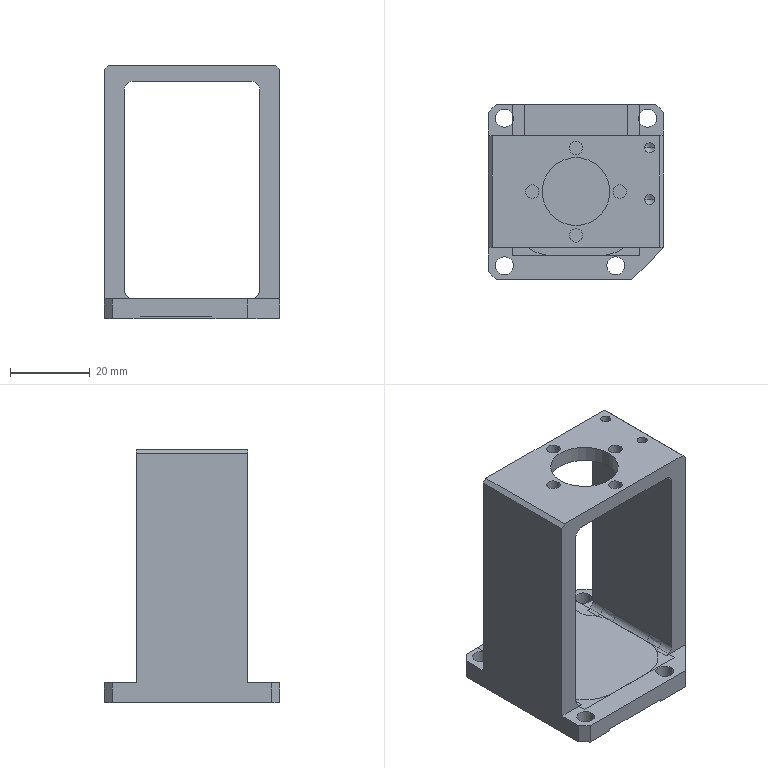NC program | NX | posted with a generic post | part box 44 x 44 x 63.6 mm
Whole program:
N10 G17 G21 G94 G90
(FLOOR_WALL_COPY , TOOL : D63)
N12 T01 M6
N14 G54
N16 G17 G0 G90 X58.5 Y0. B0. C0. S6500 M3
N18 G43 Z30. H1
N20 Z8.
N22 G94 G1 Z5. F1500.
N24 X53.5
N26 X-53.5
N28 X-58.5
N30 Z8.
N32 G0 Z30.
N34 X58.5
N36 Z7.
N38 G1 Z4.
N40 X53.5
N42 X-53.5
N44 X-58.5
N46 Z7.
N48 G0 Z30.
N50 X58.5
N52 Z6.
N54 G1 Z3.
N56 X53.5
N58 X-53.5
N60 X-58.5
N62 Z6.
N64 G0 Z30.
N66 X58.5
N68 Z5.
N70 G1 Z2.
N72 X53.5
N74 X-53.5
N76 X-58.5
N78 Z5.
N80 G0 Z30.
N82 X58.5
N84 Z4.
N86 G1 Z1.
N88 X53.5
N90 X-53.5
N92 X-58.5
N94 Z4.
N96 G0 Z30.
N98 X58.5
N100 Z3.
N102 G1 Z0.
N104 X53.5
N106 X-53.5
N108 X-58.5
N110 Z3.
N112 G0 Z30.
N114 M5
(FLOOR_WALL_1_COPY_1 , TOOL : D10)
N116 T10 M6
N118 G54
N120 G17 G0 G90 X-5.732 Y29. B0. C0. S9500 M3
N122 G43 Z30. H10
N124 Z-0.4
N126 G94 G1 X-4.866 Y27.5 F1000.
N128 G3 X-4. Y27. R1.
N130 G1 X-0.1 F2500.
N132 Y11.
N134 X-6.
N136 G3 X-8.679 Y10.222 R5.
N138 G1 X-8.684 Y10.23
N140 X-7.9 Y10.999
N142 Y27.
N144 X-4.
N146 G3 X-3.134 Y27.5 R1.
N148 G1 X-2.268 Y29.
N150 G0 Z30.
(CAVITY_MILL , TOOL : D10)
N152 X3.464 Y-27.
N154 Z1.
N156 G1 Z-0.5 F1000.
N158 X0.866 Y-22.5
N160 G3 X0. Y-22. R1.
N162 G1 Y-4.518
N164 G2 X0.4 Y-3.944 R15.6 F2500.
N166 G1 Y0.4
N168 X-0.4
N170 Y-3.944
N172 G2 X0. Y-4.518 R15.6
N174 G1 X-3.75 Y-7.006
N176 G2 X-1.9 Y-13.141 R11.1
N178 G1 Y-16.
N180 X1.9
N182 Y-13.141
N184 G2 X4.9 Y-5.552 R11.1
N186 G1 Y4.9
N188 X-4.9
N190 Y-5.552
N192 G2 X-3.75 Y-7.006 R11.1
N194 G1 X-8.75 Y-10.322
N196 G2 X-7.9 Y-13.141 R5.1
N198 G1 Y-22.
N200 X7.9
N202 Y-13.141
N204 G2 X9.43 Y-9.499 R5.1
N206 G3 X10.9 Y-6. R4.9
N208 G1 Y6.
N210 G3 X6. Y10.9 R4.9
N212 G1 X-6.
N214 X-6.764 Y10.84
N216 G3 X-10.9 Y6. R4.9
N218 G1 Y-6.
N220 G3 X-9.43 Y-9.499 R4.9
N222 G2 X-8.75 Y-10.322 R5.1
N224 G3 X-7.855 Y-10.768 R1.
N226 G1 Z1.
N228 G0 Z30.
N230 X3.464 Y-27.
N232 Z0.5
N234 G1 Z-1. F1000.
N236 X0.866 Y-22.5
N238 G3 X0. Y-22. R1.
N240 G1 Y-4.518
N242 G2 X0.4 Y-3.944 R15.6 F2500.
N244 G1 Y0.4
N246 X-0.4
N248 Y-3.944
N250 G2 X0. Y-4.518 R15.6
N252 G1 X3.75 Y-7.006
N254 G2 X4.9 Y-5.552 R11.1
N256 G1 Y4.9
N258 X-4.9
N260 Y-5.552
N262 G2 X-1.9 Y-13.141 R11.1
N264 G1 Y-16.
N266 X1.9
N268 Y-13.141
N270 G2 X3.75 Y-7.006 R11.1
N272 G1 X8.75 Y-10.322
N274 G2 X9.43 Y-9.499 R5.1
N276 G3 X10.9 Y-6. R4.9
N278 G1 Y6.
N280 G3 X6. Y10.9 R4.9
N282 G1 X-6.
N284 G3 X-10.9 Y6. R4.9
N286 G1 Y-6.
N288 G3 X-9.43 Y-9.499 R4.9
N290 G2 X-7.9 Y-13.141 R5.1
N292 G1 Y-22.
N294 X7.9
N296 Y-13.141
N298 G2 X8.75 Y-10.322 R5.1
N300 G3 X8.832 Y-10.077 R0.5
N302 G1 Z0.5
N304 G0 Z30.
N306 X3.464 Y-27.
N308 Z0.
N310 G1 Z-1.5 F1000.
N312 X0.866 Y-22.5
N314 G3 X0. Y-22. R1.
N316 G1 Y0.4
N318 X-0.4 F2500.
N320 Y-3.944
N322 G2 X0. Y-4.518 R15.6
N324 X0.4 Y-3.944 R15.6
N326 G1 Y0.4
N328 X0.
N330 Y4.9
N332 X-4.9
N334 Y-5.552
N336 G2 X-1.9 Y-13.141 R11.1
N338 G1 Y-16.
N340 X1.9
N342 Y-13.141
N344 G2 X4.9 Y-5.552 R11.1
N346 G1 Y4.9
N348 X0.
N350 Y10.9
N352 X-6.
N354 G3 X-10.9 Y6. R4.9
N356 G1 Y-6.
N358 G3 X-9.43 Y-9.499 R4.9
N360 G2 X-7.9 Y-13.141 R5.1
N362 G1 Y-22.
N364 X7.9
N366 Y-13.141
N368 G2 X9.43 Y-9.499 R5.1
N370 G3 X10.9 Y-6. R4.9
N372 G1 Y6.
N374 G3 X6. Y10.9 R4.9
N376 G1 X0.
N378 G3 X-0.866 Y10.4 R1.
N380 G1 Z0.
N382 G0 X3.464 Y-27. Z-0.5
N384 G1 Z-2. F1000.
N386 X0.866 Y-22.5
N388 G3 X0. Y-22. R1.
N390 G1 Y-4.518
N392 G2 X0.4 Y-3.944 R15.6 F2500.
N394 G1 Y0.4
N396 X-0.4
N398 Y-3.944
N400 G2 X0. Y-4.518 R15.6
N402 G1 X3.75 Y-7.006
N404 G2 X4.9 Y-5.552 R11.1
N406 G1 Y4.9
N408 X-4.9
N410 Y-5.552
N412 G2 X-1.9 Y-13.141 R11.1
N414 G1 Y-16.
N416 X1.9
N418 Y-13.141
N420 G2 X3.75 Y-7.006 R11.1
N422 G1 X8.75 Y-10.322
N424 G2 X9.43 Y-9.499 R5.1
N426 G3 X10.9 Y-6. R4.9
N428 G1 Y6.
N430 G3 X6. Y10.9 R4.9
N432 G1 X-6.
N434 G3 X-10.9 Y6. R4.9
N436 G1 Y-6.
N438 G3 X-9.43 Y-9.499 R4.9
N440 G2 X-7.9 Y-13.141 R5.1
N442 G1 Y-22.
N444 X7.9
N446 Y-13.141
N448 G2 X8.75 Y-10.322 R5.1
N450 G3 X8.832 Y-10.077 R0.5
N452 G1 Z-0.5
N454 G0 Z30.
N456 X3.464 Y-27.
N458 Z-1.
N460 G1 Z-2.5 F1000.
N462 X0.866 Y-22.5
N464 G3 X0. Y-22. R1.
N466 G1 Y-4.518
N468 G2 X0.4 Y-3.944 R15.6 F2500.
N470 G1 Y0.4
N472 X-0.4
N474 Y-3.944
N476 G2 X0. Y-4.518 R15.6
N478 G1 X-3.75 Y-7.006
N480 G2 X-1.9 Y-13.141 R11.1
N482 G1 Y-16.
N484 X1.9
N486 Y-13.141
N488 G2 X4.9 Y-5.552 R11.1
N490 G1 Y4.9
N492 X-4.9
N494 Y-5.552
N496 G2 X-3.75 Y-7.006 R11.1
N498 G1 X-8.75 Y-10.322
N500 G2 X-7.9 Y-13.141 R5.1
N502 G1 Y-22.
N504 X7.9
N506 Y-13.141
N508 G2 X9.43 Y-9.499 R5.1
N510 G3 X10.9 Y-6. R4.9
N512 G1 Y6.
N514 G3 X6. Y10.9 R4.9
N516 G1 X-6.
N518 G3 X-10.9 Y6. R4.9
N520 G1 Y-6.
N522 G3 X-9.43 Y-9.499 R4.9
N524 G2 X-8.75 Y-10.322 R5.1
N526 G3 X-7.855 Y-10.768 R1.
N528 G1 Z-1.
N530 G0 X3.464 Y-27. Z-1.5
N532 G1 Z-3. F1000.
N534 X0.866 Y-22.5
N536 G3 X0. Y-22. R1.
N538 G1 Y-4.518
N540 G2 X0.4 Y-3.944 R15.6 F2500.
N542 G1 Y0.4
N544 X-0.4
N546 Y-3.944
N548 G2 X0. Y-4.518 R15.6
N550 G1 X-3.75 Y-7.006
N552 G2 X-1.9 Y-13.141 R11.1
N554 G1 Y-16.
N556 X1.9
N558 Y-13.141
N560 G2 X4.9 Y-5.552 R11.1
N562 G1 Y4.9
N564 X-4.9
N566 Y-5.552
N568 G2 X-3.75 Y-7.006 R11.1
N570 G1 X-8.75 Y-10.322
N572 G2 X-7.9 Y-13.141 R5.1
N574 G1 Y-22.
N576 X7.9
N578 Y-13.141
N580 G2 X9.43 Y-9.499 R5.1
N582 G3 X10.9 Y-6. R4.9
N584 G1 Y6.
N586 G3 X6. Y10.9 R4.9
N588 G1 X-6.
N590 G3 X-10.9 Y6. R4.9
N592 G1 Y-6.
N594 G3 X-9.43 Y-9.499 R4.9
N596 G2 X-8.75 Y-10.322 R5.1
N598 G3 X-7.855 Y-10.768 R1.
N600 G1 Z-1.5
N602 G0 X3.464 Y-27. Z-2.
N604 G1 Z-3.5 F1000.
N606 X0.866 Y-22.5
N608 G3 X0. Y-22. R1.
N610 G1 Y-4.518
N612 G2 X0.4 Y-3.944 R15.6 F2500.
N614 G1 Y0.4
N616 X-0.4
N618 Y-3.944
N620 G2 X0. Y-4.518 R15.6
N622 G1 X3.75 Y-7.006
N624 G2 X4.9 Y-5.552 R11.1
N626 G1 Y4.9
N628 X-4.9
N630 Y-5.552
N632 G2 X-1.9 Y-13.141 R11.1
N634 G1 Y-16.
N636 X1.9
N638 Y-13.141
N640 G2 X3.75 Y-7.006 R11.1
N642 G1 X8.75 Y-10.322
N644 G2 X9.43 Y-9.499 R5.1
N646 G3 X10.9 Y-6. R4.9
N648 G1 Y6.
N650 G3 X6. Y10.9 R4.9
N652 G1 X-6.
N654 G3 X-10.9 Y6. R4.9
N656 G1 Y-6.
N658 G3 X-9.43 Y-9.499 R4.9
N660 G2 X-7.9 Y-13.141 R5.1
N662 G1 Y-22.
N664 X7.9
N666 Y-13.141
N668 G2 X8.75 Y-10.322 R5.1
N670 G3 X8.832 Y-10.077 R0.5
N672 G1 Z-2.
N674 G0 Z30.
N676 X3.464 Y-27.
N678 Z-2.5
N680 G1 Z-4. F1000.
N682 X0.866 Y-22.5
N684 G3 X0. Y-22. R1.
N686 G1 Y-4.518
N688 G2 X0.4 Y-3.944 R15.6 F2500.
N690 G1 Y0.4
N692 X-0.4
N694 Y-3.944
N696 G2 X0. Y-4.518 R15.6
N698 G1 X3.75 Y-7.006
N700 G2 X4.9 Y-5.552 R11.1
N702 G1 Y4.9
N704 X-4.9
N706 Y-5.552
N708 G2 X-1.9 Y-13.141 R11.1
N710 G1 Y-16.
N712 X1.9
N714 Y-13.141
N716 G2 X3.75 Y-7.006 R11.1
N718 G1 X8.75 Y-10.322
N720 G2 X9.43 Y-9.499 R5.1
N722 G3 X10.9 Y-6. R4.9
N724 G1 Y6.
N726 G3 X6. Y10.9 R4.9
N728 G1 X-6.
N730 G3 X-10.9 Y6. R4.9
N732 G1 Y-6.
N734 G3 X-9.43 Y-9.499 R4.9
N736 G2 X-7.9 Y-13.141 R5.1
N738 G1 Y-22.
N740 X7.9
N742 Y-13.141
N744 G2 X8.75 Y-10.322 R5.1
N746 G3 X8.832 Y-10.077 R0.5
N748 G1 Z-2.5
N750 G0 Z30.
N752 X3.464 Y-27.
N754 Z-3.
N756 G1 Z-4.5 F1000.
N758 X0.866 Y-22.5
N760 G3 X0. Y-22. R1.
N762 G1 Y0.4
N764 X-0.4 F2500.
N766 Y-3.944
N768 G2 X0. Y-4.518 R15.6
N770 X0.4 Y-3.944 R15.6
N772 G1 Y0.4
N774 X0.
N776 Y4.9
N778 X-4.9
N780 Y-5.552
N782 G2 X-1.9 Y-13.141 R11.1
N784 G1 Y-16.
N786 X1.9
N788 Y-13.141
N790 G2 X4.9 Y-5.552 R11.1
N792 G1 Y4.9
N794 X0.
N796 Y10.9
N798 X-6.
N800 G3 X-10.9 Y6. R4.9
N802 G1 Y-6.
N804 G3 X-9.43 Y-9.499 R4.9
N806 G2 X-7.9 Y-13.141 R5.1
N808 G1 Y-22.
N810 X7.9
N812 Y-13.141
N814 G2 X9.43 Y-9.499 R5.1
N816 G3 X10.9 Y-6. R4.9
N818 G1 Y6.
N820 G3 X6. Y10.9 R4.9
N822 G1 X0.
N824 G3 X-0.866 Y10.4 R1.
N826 G1 Z-3.
N828 G0 X3.464 Y-27. Z-3.5
N830 G1 Z-5. F1000.
N832 X0.866 Y-22.5
N834 G3 X0. Y-22. R1.
N836 G1 Y-4.518
N838 G2 X0.4 Y-3.944 R15.6 F2500.
N840 G1 Y0.4
N842 X-0.4
N844 Y-3.944
N846 G2 X0. Y-4.518 R15.6
N848 G1 X-3.75 Y-7.006
N850 G2 X-1.9 Y-13.141 R11.1
N852 G1 Y-16.
N854 X1.9
N856 Y-13.141
N858 G2 X4.9 Y-5.552 R11.1
N860 G1 Y4.9
N862 X-4.9
N864 Y-5.552
N866 G2 X-3.75 Y-7.006 R11.1
N868 G1 X-8.75 Y-10.322
N870 G2 X-7.9 Y-13.141 R5.1
N872 G1 Y-22.
N874 X7.9
N876 Y-13.141
N878 G2 X9.43 Y-9.499 R5.1
N880 G3 X10.9 Y-6. R4.9
N882 G1 Y6.
N884 G3 X6. Y10.9 R4.9
N886 G1 X-6.
N888 G3 X-10.9 Y6. R4.9
N890 G1 Y-6.
N892 G3 X-9.43 Y-9.499 R4.9
N894 G2 X-8.75 Y-10.322 R5.1
N896 G3 X-7.855 Y-10.768 R1.
N898 G1 Z-3.5
N900 G0 Z30.
N902 M5
(ZLEVEL_PROFILE_1 , TOOL : D10JING)
N904 T11 M6
N906 G54
N908 G17 G0 G90 X6.081 Y-28.514 B0. C0. S9500 M3
N910 G43 Z30. H11
N912 Z-3.5
N914 G94 G1 Z-5. F1250.
N916 X7.502 Y-27.692
N918 G3 X8.002 Y-26.826 R1.
N920 G1 X8. Y-22.054
N922 Y-13.141
N924 G2 X9.5 Y-9.571 R5.
N926 G3 X11. Y-6. R5.
N928 G1 Y6.
N930 G3 X6. Y11. R5.
N932 G1 X-6.
N934 G3 X-11. Y6. R5.
N936 G1 Y-6.
N938 G3 X-9.5 Y-9.571 R5.
N940 G2 X-8. Y-13.141 R5.
N942 G1 Y-22.
N944 X-8.025 Y-22.501
N946 X-8.002 Y-22.551
N948 Y-26.826
N950 G3 X-7.502 Y-27.692 R1.
N952 G1 X-6.081 Y-28.512
N954 Z-3.5
N956 G0 Z30.
N958 M5
(DRILLING_COPY_1 , TOOL : D6A45)
N960 T07 M6
N962 G54
N964 G17 G0 G90 X-18. Y-18.5 B0. C0. S5000 M3
N966 G43 Z30. H7
N968 G94 G81 G98 Z-1.6 F250. R3.
N970 Y18.5
N972 X18. Y-18.5
N974 X10. Y18.5
N976 G80
N978 G0 X10. Y18.5 Z30.
N980 M5
(DRILLING_COPY_2 , TOOL : 4.5ZT)
N982 T14 M6
N984 G54
N986 G17 G0 G90 X-18. Y-18.5 B0. C0. S2000 M3
N988 G43 Z30. H14
N990 G94 G83 G98 Z-7.852 F250. Q2. R3.
N992 Y18.5
N994 X18. Y-18.5
N996 X10. Y18.5
N998 G80
N1000 G0 X10. Y18.5 Z30.
N1002 M5
(PLANAR_MILL_COPY_1_COPY , TOOL : D6A45)
N1004 T07 M6
N1006 G54
N1008 G17 G0 G90 X-18.85 Y18.632 B0. C0. S9500 M3
N1010 G43 Z30. H7
N1012 Z0.
N1014 G94 G1 Y18.272 Z-0.096 F1250.
N1016 X-18.622 Y17.878 Z-0.218
N1018 X-18.228 Y17.65 Z-0.34
N1020 X-17.772 Z-0.463
N1022 X-17.378 Y17.878 Z-0.585
N1024 X-17.15 Y18.272 Z-0.707
N1026 Y18.728 Z-0.829
N1028 X-17.378 Y19.122 Z-0.951
N1030 X-17.772 Y19.35 Z-1.073
N1032 X-18.228 Z-1.195
N1034 X-18.622 Y19.122 Z-1.317
N1036 X-18.85 Y18.728 Z-1.439
N1038 Y18.5 Z-1.5
N1040 G3 X-18. Y17.65 R0.85
N1042 X-18.85 Y18.5 R-0.85
N1044 X-18.6 Y18.067 R0.5
N1046 G1 Z0.
N1048 G0 Z30.
N1050 X10.132 Y19.35
N1052 Z0.
N1054 G1 X9.772 Z-0.096
N1056 X9.378 Y19.122 Z-0.218
N1058 X9.15 Y18.728 Z-0.34
N1060 Y18.272 Z-0.463
N1062 X9.378 Y17.878 Z-0.585
N1064 X9.772 Y17.65 Z-0.707
N1066 X10.228 Z-0.829
N1068 X10.622 Y17.878 Z-0.951
N1070 X10.85 Y18.272 Z-1.073
N1072 Y18.728 Z-1.195
N1074 X10.622 Y19.122 Z-1.317
N1076 X10.228 Y19.35 Z-1.439
N1078 X10. Z-1.5
N1080 G3 X9.15 Y18.5 R0.85
N1082 X10. Y19.35 R-0.85
N1084 X9.567 Y19.1 R0.5
N1086 G1 Z0.
N1088 G0 Z30.
N1090 X4.827 Y24.7
N1092 Z0.
N1094 G1 Z-1.5
N1096 X4.91 Y24.178
N1098 G3 X5.539 Y23.4 R1.
N1100 G1 X13.959
N1102 G2 X15.019 Y22.961 R1.5
N1104 G1 X22.961 Y15.019
N1106 G2 X23.4 Y13.959 R1.5
N1108 G1 Y-19.959
N1110 G2 X22.961 Y-21.019 R1.5
N1112 G1 X21.019 Y-22.961
N1114 G2 X19.959 Y-23.4 R1.5
N1116 G1 X13.1
N1118 G2 X11.6 Y-21.9 R1.5
N1120 G1 Y-13.183
N1122 G2 X12.046 Y-12.116 R1.5
N1124 G3 X14.6 Y-6. R8.6
N1126 G1 Y6.
N1128 G3 X6. Y14.6 R8.6
N1130 G1 X5.539
N1132 G3 X4.91 Y13.822 R1.
N1134 G1 X4.827 Y13.3
N1136 Z0.
N1138 G0 Z30.
N1140 X-10.929 Y11.385
N1142 Z0.
N1144 G1 Z-1.5
N1146 X-11.37 Y11.694
N1148 G3 X-12.366 Y11.782 R1.
N1150 X-14.6 Y6. R8.6
N1152 G1 Y-6.
N1154 G3 X-12.046 Y-12.116 R8.6
N1156 G2 X-11.6 Y-13.183 R1.5
N1158 G1 Y-21.9
N1160 G2 X-13.1 Y-23.4 R1.5
N1162 G1 X-19.959
N1164 G2 X-21.019 Y-22.961 R1.5
N1166 G1 X-22.961 Y-21.019
N1168 G2 X-23.4 Y-19.959 R1.5
N1170 G1 Y19.959
N1172 G2 X-22.961 Y21.019 R1.5
N1174 G1 X-21.019 Y22.961
N1176 G2 X-19.959 Y23.4 R1.5
N1178 G1 X-13.539
N1180 G3 X-12.91 Y24.178 R1.
N1182 G1 X-12.827 Y24.7
N1184 Z0.
N1186 G0 Z30.
N1188 X17.868 Y-19.35
N1190 Z0.
N1192 G1 X18.228 Z-0.096
N1194 X18.622 Y-19.122 Z-0.218
N1196 X18.85 Y-18.728 Z-0.34
N1198 Y-18.272 Z-0.463
N1200 X18.622 Y-17.878 Z-0.585
N1202 X18.228 Y-17.65 Z-0.707
N1204 X17.772 Z-0.829
N1206 X17.378 Y-17.878 Z-0.951
N1208 X17.15 Y-18.272 Z-1.073
N1210 Y-18.728 Z-1.195
N1212 X17.378 Y-19.122 Z-1.317
N1214 X17.772 Y-19.35 Z-1.439
N1216 X18. Z-1.5
N1218 G3 X18.85 Y-18.5 R0.85
N1220 X18. Y-19.35 R-0.85
N1222 X18.433 Y-19.1 R0.5
N1224 G1 Z0.
N1226 G0 Z30.
N1228 X-18.132 Y-19.35
N1230 Z0.
N1232 G1 X-17.772 Z-0.096
N1234 X-17.378 Y-19.122 Z-0.218
N1236 X-17.15 Y-18.728 Z-0.34
N1238 Y-18.272 Z-0.463
N1240 X-17.378 Y-17.878 Z-0.585
N1242 X-17.772 Y-17.65 Z-0.707
N1244 X-18.228 Z-0.829
N1246 X-18.622 Y-17.878 Z-0.951
N1248 X-18.85 Y-18.272 Z-1.073
N1250 Y-18.728 Z-1.195
N1252 X-18.622 Y-19.122 Z-1.317
N1254 X-18.228 Y-19.35 Z-1.439
N1256 X-18. Z-1.5
N1258 G3 X-17.15 Y-18.5 R0.85
N1260 X-18. Y-19.35 R-0.85
N1262 X-17.567 Y-19.1 R0.5
N1264 G1 Z0.
N1266 G0 Z30.
(PLANAR_MILL_COPY_1_COPY_COPY , TOOL : D6A45)
N1268 X2.74 Y13.07
N1270 Z-0.5
N1272 G1 Z-2.
N1274 X2.999 Y13.603
N1276 G3 X2.929 Y14.6 R1.
N1278 G1 X-6.
N1280 G3 X-10.5 Y13.329 R8.6
N1282 X-10. Y12.463 R1.
N1284 G1 X-9.439 Y12.139
N1286 Z-0.5
N1288 G0 Z30.
N1290 X-10.74 Y24.93
N1292 Z-0.5
N1294 G1 Z-2.
N1296 X-10.999 Y24.397
N1298 G3 X-10.929 Y23.4 R1.
N1300 G1 X2.929
N1302 G3 X2.999 Y24.397 R1.
N1304 G1 X2.74 Y24.93
N1306 Z-0.5
N1308 G0 Z30.
N1310 M5
N1312 M2